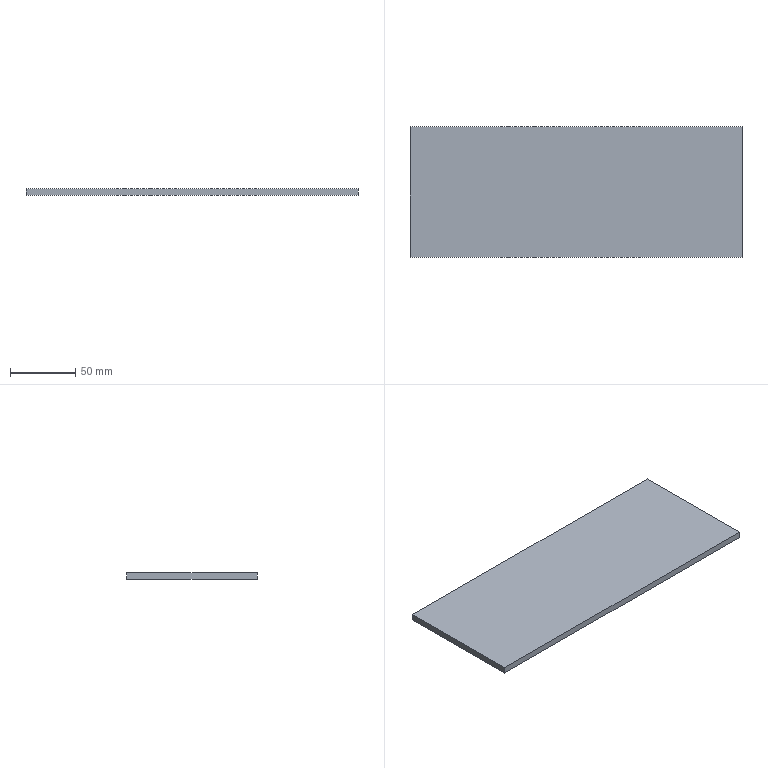Part | SolidWorks | features ICE 3, Extrusion 1 | 1 solid | 6 faces | box 255 x 100 x 5 mm | volume 127500 mm3 | plane 6
STEP:
#1=CARTESIAN_POINT('',(0.,0.,-5.));
#2=VERTEX_POINT('',#1);
#3=CARTESIAN_POINT('',(255.,0.,-5.));
#4=VERTEX_POINT('',#3);
#5=CARTESIAN_POINT('',(0.,0.,-5.));
#6=DIRECTION('',(1.,0.,0.));
#7=VECTOR('',#6,1000.);
#8=LINE('',#5,#7);
#9=EDGE_CURVE('',#2,#4,#8,.T.);
#10=ORIENTED_EDGE('',*,*,#9,.F.);
#11=CARTESIAN_POINT('',(0.,100.,-5.));
#12=VERTEX_POINT('',#11);
#13=CARTESIAN_POINT('',(0.,100.,-5.));
#14=DIRECTION('',(0.,-1.,0.));
#15=VECTOR('',#14,1000.);
#16=LINE('',#13,#15);
#17=EDGE_CURVE('',#12,#2,#16,.T.);
#18=ORIENTED_EDGE('',*,*,#17,.F.);
#19=CARTESIAN_POINT('',(255.,100.,-5.));
#20=VERTEX_POINT('',#19);
#21=CARTESIAN_POINT('',(255.,100.,-5.));
#22=DIRECTION('',(-1.,0.,0.));
#23=VECTOR('',#22,1000.);
#24=LINE('',#21,#23);
#25=EDGE_CURVE('',#20,#12,#24,.T.);
#26=ORIENTED_EDGE('',*,*,#25,.F.);
#27=CARTESIAN_POINT('',(255.,0.,-5.));
#28=DIRECTION('',(0.,1.,0.));
#29=VECTOR('',#28,1000.);
#30=LINE('',#27,#29);
#31=EDGE_CURVE('',#4,#20,#30,.T.);
#32=ORIENTED_EDGE('',*,*,#31,.F.);
#33=EDGE_LOOP('',(#10,#18,#26,#32));
#34=FACE_OUTER_BOUND('',#33,.T.);
#35=CARTESIAN_POINT('',(0.,0.,-5.));
#36=DIRECTION('',(0.,0.,1.));
#37=DIRECTION('',(1.,0.,0.));
#38=AXIS2_PLACEMENT_3D('',#35,#36,#37);
#39=PLANE('',#38);
#40=ADVANCED_FACE('',(#34),#39,.F.);
#41=CARTESIAN_POINT('',(0.,100.,0.));
#42=VERTEX_POINT('',#41);
#43=CARTESIAN_POINT('',(0.,0.,0.));
#44=VERTEX_POINT('',#43);
#45=CARTESIAN_POINT('',(0.,100.,0.));
#46=DIRECTION('',(0.,-1.,0.));
#47=VECTOR('',#46,1000.);
#48=LINE('',#45,#47);
#49=EDGE_CURVE('',#42,#44,#48,.T.);
#50=ORIENTED_EDGE('',*,*,#49,.T.);
#51=CARTESIAN_POINT('',(255.,0.,0.));
#52=VERTEX_POINT('',#51);
#53=CARTESIAN_POINT('',(0.,0.,0.));
#54=DIRECTION('',(1.,0.,0.));
#55=VECTOR('',#54,1000.);
#56=LINE('',#53,#55);
#57=EDGE_CURVE('',#44,#52,#56,.T.);
#58=ORIENTED_EDGE('',*,*,#57,.T.);
#59=CARTESIAN_POINT('',(255.,100.,0.));
#60=VERTEX_POINT('',#59);
#61=CARTESIAN_POINT('',(255.,0.,0.));
#62=DIRECTION('',(0.,1.,0.));
#63=VECTOR('',#62,1000.);
#64=LINE('',#61,#63);
#65=EDGE_CURVE('',#52,#60,#64,.T.);
#66=ORIENTED_EDGE('',*,*,#65,.T.);
#67=CARTESIAN_POINT('',(255.,100.,0.));
#68=DIRECTION('',(-1.,0.,0.));
#69=VECTOR('',#68,1000.);
#70=LINE('',#67,#69);
#71=EDGE_CURVE('',#60,#42,#70,.T.);
#72=ORIENTED_EDGE('',*,*,#71,.T.);
#73=EDGE_LOOP('',(#50,#58,#66,#72));
#74=FACE_OUTER_BOUND('',#73,.T.);
#75=CARTESIAN_POINT('',(0.,0.,0.));
#76=DIRECTION('',(0.,0.,1.));
#77=DIRECTION('',(1.,0.,0.));
#78=AXIS2_PLACEMENT_3D('',#75,#76,#77);
#79=PLANE('',#78);
#80=ADVANCED_FACE('',(#74),#79,.T.);
#81=ORIENTED_EDGE('',*,*,#17,.T.);
#82=CARTESIAN_POINT('',(0.,0.,0.));
#83=DIRECTION('',(0.,0.,-1.));
#84=VECTOR('',#83,1000.);
#85=LINE('',#82,#84);
#86=EDGE_CURVE('',#44,#2,#85,.T.);
#87=ORIENTED_EDGE('',*,*,#86,.F.);
#88=ORIENTED_EDGE('',*,*,#49,.F.);
#89=CARTESIAN_POINT('',(0.,100.,0.));
#90=DIRECTION('',(0.,0.,-1.));
#91=VECTOR('',#90,1000.);
#92=LINE('',#89,#91);
#93=EDGE_CURVE('',#42,#12,#92,.T.);
#94=ORIENTED_EDGE('',*,*,#93,.T.);
#95=EDGE_LOOP('',(#81,#87,#88,#94));
#96=FACE_OUTER_BOUND('',#95,.T.);
#97=CARTESIAN_POINT('',(0.,100.,-5.));
#98=DIRECTION('',(-1.,0.,0.));
#99=DIRECTION('',(0.,0.,1.));
#100=AXIS2_PLACEMENT_3D('',#97,#98,#99);
#101=PLANE('',#100);
#102=ADVANCED_FACE('',(#96),#101,.T.);
#103=ORIENTED_EDGE('',*,*,#71,.F.);
#104=CARTESIAN_POINT('',(255.,100.,0.));
#105=DIRECTION('',(0.,0.,-1.));
#106=VECTOR('',#105,1000.);
#107=LINE('',#104,#106);
#108=EDGE_CURVE('',#60,#20,#107,.T.);
#109=ORIENTED_EDGE('',*,*,#108,.T.);
#110=ORIENTED_EDGE('',*,*,#25,.T.);
#111=ORIENTED_EDGE('',*,*,#93,.F.);
#112=EDGE_LOOP('',(#103,#109,#110,#111));
#113=FACE_OUTER_BOUND('',#112,.T.);
#114=CARTESIAN_POINT('',(255.,100.,-5.));
#115=DIRECTION('',(0.,1.,0.));
#116=DIRECTION('',(0.,0.,1.));
#117=AXIS2_PLACEMENT_3D('',#114,#115,#116);
#118=PLANE('',#117);
#119=ADVANCED_FACE('',(#113),#118,.T.);
#120=ORIENTED_EDGE('',*,*,#65,.F.);
#121=CARTESIAN_POINT('',(255.,0.,0.));
#122=DIRECTION('',(0.,0.,-1.));
#123=VECTOR('',#122,1000.);
#124=LINE('',#121,#123);
#125=EDGE_CURVE('',#52,#4,#124,.T.);
#126=ORIENTED_EDGE('',*,*,#125,.T.);
#127=ORIENTED_EDGE('',*,*,#31,.T.);
#128=ORIENTED_EDGE('',*,*,#108,.F.);
#129=EDGE_LOOP('',(#120,#126,#127,#128));
#130=FACE_OUTER_BOUND('',#129,.T.);
#131=CARTESIAN_POINT('',(255.,0.,-5.));
#132=DIRECTION('',(1.,0.,0.));
#133=DIRECTION('',(0.,0.,-1.));
#134=AXIS2_PLACEMENT_3D('',#131,#132,#133);
#135=PLANE('',#134);
#136=ADVANCED_FACE('',(#130),#135,.T.);
#137=ORIENTED_EDGE('',*,*,#57,.F.);
#138=ORIENTED_EDGE('',*,*,#86,.T.);
#139=ORIENTED_EDGE('',*,*,#9,.T.);
#140=ORIENTED_EDGE('',*,*,#125,.F.);
#141=EDGE_LOOP('',(#137,#138,#139,#140));
#142=FACE_OUTER_BOUND('',#141,.T.);
#143=CARTESIAN_POINT('',(0.,0.,-5.));
#144=DIRECTION('',(0.,-1.,0.));
#145=DIRECTION('',(0.,0.,-1.));
#146=AXIS2_PLACEMENT_3D('',#143,#144,#145);
#147=PLANE('',#146);
#148=ADVANCED_FACE('',(#142),#147,.T.);
#149=CLOSED_SHELL('',(#40,#80,#102,#119,#136,#148));
#150=MANIFOLD_SOLID_BREP('',#149);
#151=CARTESIAN_POINT('',(0.,0.,0.));
#152=DIRECTION('',(0.,0.,1.));
#153=DIRECTION('',(1.,0.,0.));
#154=AXIS2_PLACEMENT_3D('',#151,#152,#153);
#155=(LENGTH_UNIT()NAMED_UNIT(*)SI_UNIT(.MILLI.,.METRE.));
#156=UNCERTAINTY_MEASURE_WITH_UNIT(LENGTH_MEASURE(0.00001),#155,'','');
#157=(NAMED_UNIT(*)PLANE_ANGLE_UNIT()SI_UNIT($,.RADIAN.));
#158=(NAMED_UNIT(*)SI_UNIT($,.STERADIAN.)SOLID_ANGLE_UNIT());
#159=(GEOMETRIC_REPRESENTATION_CONTEXT(3)GLOBAL_UNCERTAINTY_ASSIGNED_CONTEXT((#156))GLOBAL_UNIT_ASSIGNED_CONTEXT((#155,#157,#158))REPRESENTATION_CONTEXT('',''));
#160=ADVANCED_BREP_SHAPE_REPRESENTATION('',(#150,#154),#159);